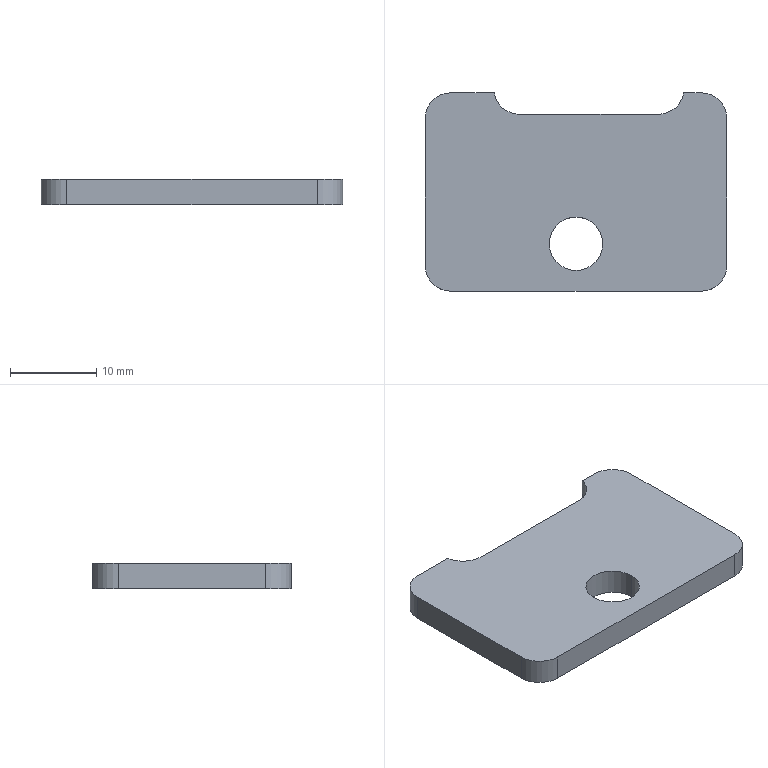Part | SolidWorks | features Fillet 2, MoveFace 2, Extrusion 1, ICE 1 | 1 solid | 16 faces | box 35 x 23 x 3 mm | volume 2147 mm3 | cylinder 8 | plane 8 | commonest cylinder face diameters 6 x6 6.2 x2
STEP:
#1=CARTESIAN_POINT('',(-3.1,-7.,3.));
#2=VERTEX_POINT('',#1);
#3=CARTESIAN_POINT('',(3.1,-7.,3.));
#4=VERTEX_POINT('',#3);
#5=CARTESIAN_POINT('',(0.,-7.,3.));
#6=DIRECTION('',(0.,0.,1.));
#7=DIRECTION('',(1.,0.,0.));
#8=AXIS2_PLACEMENT_3D('',#5,#6,#7);
#9=CIRCLE('',#8,3.1);
#10=EDGE_CURVE('',#2,#4,#9,.T.);
#11=ORIENTED_EDGE('',*,*,#10,.T.);
#12=CARTESIAN_POINT('',(3.1,-7.,0.));
#13=VERTEX_POINT('',#12);
#14=CARTESIAN_POINT('',(3.1,-7.,3.));
#15=DIRECTION('',(0.,0.,-1.));
#16=VECTOR('',#15,1000.);
#17=LINE('',#14,#16);
#18=EDGE_CURVE('',#4,#13,#17,.T.);
#19=ORIENTED_EDGE('',*,*,#18,.T.);
#20=CARTESIAN_POINT('',(-3.1,-7.,0.));
#21=VERTEX_POINT('',#20);
#22=CARTESIAN_POINT('',(0.,-7.,0.));
#23=DIRECTION('',(0.,0.,1.));
#24=DIRECTION('',(1.,0.,0.));
#25=AXIS2_PLACEMENT_3D('',#22,#23,#24);
#26=CIRCLE('',#25,3.1);
#27=EDGE_CURVE('',#21,#13,#26,.T.);
#28=ORIENTED_EDGE('',*,*,#27,.F.);
#29=CARTESIAN_POINT('',(-3.1,-7.,3.));
#30=DIRECTION('',(0.,0.,-1.));
#31=VECTOR('',#30,1000.);
#32=LINE('',#29,#31);
#33=EDGE_CURVE('',#2,#21,#32,.T.);
#34=ORIENTED_EDGE('',*,*,#33,.F.);
#35=EDGE_LOOP('',(#11,#19,#28,#34));
#36=FACE_OUTER_BOUND('',#35,.T.);
#37=CARTESIAN_POINT('',(0.,-7.,3.));
#38=DIRECTION('',(0.,0.,-1.));
#39=DIRECTION('',(-1.,0.,0.));
#40=AXIS2_PLACEMENT_3D('',#37,#38,#39);
#41=CYLINDRICAL_SURFACE('',#40,3.1);
#42=ADVANCED_FACE('',(#36),#41,.F.);
#43=CARTESIAN_POINT('',(-9.5,10.5,3.));
#44=VERTEX_POINT('',#43);
#45=CARTESIAN_POINT('',(-14.5,10.5,3.));
#46=VERTEX_POINT('',#45);
#47=CARTESIAN_POINT('',(-17.5,10.5,3.));
#48=DIRECTION('',(-1.,0.,0.));
#49=VECTOR('',#48,1000.);
#50=LINE('',#47,#49);
#51=EDGE_CURVE('',#44,#46,#50,.T.);
#52=ORIENTED_EDGE('',*,*,#51,.F.);
#53=CARTESIAN_POINT('',(-9.5,10.5,0.));
#54=VERTEX_POINT('',#53);
#55=CARTESIAN_POINT('',(-9.5,10.5,3.));
#56=DIRECTION('',(0.,0.,-1.));
#57=VECTOR('',#56,1000.);
#58=LINE('',#55,#57);
#59=EDGE_CURVE('',#44,#54,#58,.T.);
#60=ORIENTED_EDGE('',*,*,#59,.T.);
#61=CARTESIAN_POINT('',(-14.5,10.5,0.));
#62=VERTEX_POINT('',#61);
#63=CARTESIAN_POINT('',(-17.5,10.5,0.));
#64=DIRECTION('',(-1.,0.,0.));
#65=VECTOR('',#64,1000.);
#66=LINE('',#63,#65);
#67=EDGE_CURVE('',#54,#62,#66,.T.);
#68=ORIENTED_EDGE('',*,*,#67,.T.);
#69=CARTESIAN_POINT('',(-14.5,10.5,3.));
#70=DIRECTION('',(0.,0.,1.));
#71=VECTOR('',#70,1000.);
#72=LINE('',#69,#71);
#73=EDGE_CURVE('',#62,#46,#72,.T.);
#74=ORIENTED_EDGE('',*,*,#73,.T.);
#75=EDGE_LOOP('',(#52,#60,#68,#74));
#76=FACE_OUTER_BOUND('',#75,.T.);
#77=CARTESIAN_POINT('',(-17.5,10.5,3.));
#78=DIRECTION('',(0.,-1.,0.));
#79=DIRECTION('',(0.,0.,-1.));
#80=AXIS2_PLACEMENT_3D('',#77,#78,#79);
#81=PLANE('',#80);
#82=ADVANCED_FACE('',(#76),#81,.F.);
#83=CARTESIAN_POINT('',(9.542,8.,3.));
#84=VERTEX_POINT('',#83);
#85=CARTESIAN_POINT('',(-6.542,8.,3.));
#86=VERTEX_POINT('',#85);
#87=CARTESIAN_POINT('',(12.5,8.,3.));
#88=DIRECTION('',(-1.,0.,0.));
#89=VECTOR('',#88,1000.);
#90=LINE('',#87,#89);
#91=EDGE_CURVE('',#84,#86,#90,.T.);
#92=ORIENTED_EDGE('',*,*,#91,.T.);
#93=CARTESIAN_POINT('',(-6.542,11.,3.));
#94=DIRECTION('',(0.,0.,-1.));
#95=DIRECTION('',(1.,0.,0.));
#96=AXIS2_PLACEMENT_3D('',#93,#94,#95);
#97=CIRCLE('',#96,3.);
#98=EDGE_CURVE('',#86,#44,#97,.T.);
#99=ORIENTED_EDGE('',*,*,#98,.T.);
#100=ORIENTED_EDGE('',*,*,#51,.T.);
#101=CARTESIAN_POINT('',(-17.5,7.5,3.));
#102=VERTEX_POINT('',#101);
#103=CARTESIAN_POINT('',(-14.5,7.5,3.));
#104=DIRECTION('',(0.,0.,1.));
#105=DIRECTION('',(1.,0.,0.));
#106=AXIS2_PLACEMENT_3D('',#103,#104,#105);
#107=CIRCLE('',#106,3.);
#108=EDGE_CURVE('',#46,#102,#107,.T.);
#109=ORIENTED_EDGE('',*,*,#108,.T.);
#110=CARTESIAN_POINT('',(-17.5,-9.5,3.));
#111=VERTEX_POINT('',#110);
#112=CARTESIAN_POINT('',(-17.5,12.5,3.));
#113=DIRECTION('',(0.,-1.,0.));
#114=VECTOR('',#113,1000.);
#115=LINE('',#112,#114);
#116=EDGE_CURVE('',#102,#111,#115,.T.);
#117=ORIENTED_EDGE('',*,*,#116,.T.);
#118=CARTESIAN_POINT('',(-14.5,-12.5,3.));
#119=VERTEX_POINT('',#118);
#120=CARTESIAN_POINT('',(-14.5,-9.5,3.));
#121=DIRECTION('',(0.,0.,1.));
#122=DIRECTION('',(1.,0.,0.));
#123=AXIS2_PLACEMENT_3D('',#120,#121,#122);
#124=CIRCLE('',#123,3.);
#125=EDGE_CURVE('',#111,#119,#124,.T.);
#126=ORIENTED_EDGE('',*,*,#125,.T.);
#127=CARTESIAN_POINT('',(14.5,-12.5,3.));
#128=VERTEX_POINT('',#127);
#129=CARTESIAN_POINT('',(-17.5,-12.5,3.));
#130=DIRECTION('',(1.,0.,0.));
#131=VECTOR('',#130,1000.);
#132=LINE('',#129,#131);
#133=EDGE_CURVE('',#119,#128,#132,.T.);
#134=ORIENTED_EDGE('',*,*,#133,.T.);
#135=CARTESIAN_POINT('',(17.5,-9.5,3.));
#136=VERTEX_POINT('',#135);
#137=CARTESIAN_POINT('',(14.5,-9.5,3.));
#138=DIRECTION('',(0.,0.,1.));
#139=DIRECTION('',(1.,0.,0.));
#140=AXIS2_PLACEMENT_3D('',#137,#138,#139);
#141=CIRCLE('',#140,3.);
#142=EDGE_CURVE('',#128,#136,#141,.T.);
#143=ORIENTED_EDGE('',*,*,#142,.T.);
#144=CARTESIAN_POINT('',(17.5,7.5,3.));
#145=VERTEX_POINT('',#144);
#146=CARTESIAN_POINT('',(17.5,12.5,3.));
#147=DIRECTION('',(0.,1.,0.));
#148=VECTOR('',#147,1000.);
#149=LINE('',#146,#148);
#150=EDGE_CURVE('',#136,#145,#149,.T.);
#151=ORIENTED_EDGE('',*,*,#150,.T.);
#152=CARTESIAN_POINT('',(14.5,10.5,3.));
#153=VERTEX_POINT('',#152);
#154=CARTESIAN_POINT('',(14.5,7.5,3.));
#155=DIRECTION('',(0.,0.,1.));
#156=DIRECTION('',(1.,0.,0.));
#157=AXIS2_PLACEMENT_3D('',#154,#155,#156);
#158=CIRCLE('',#157,3.);
#159=EDGE_CURVE('',#145,#153,#158,.T.);
#160=ORIENTED_EDGE('',*,*,#159,.T.);
#161=CARTESIAN_POINT('',(12.5,10.5,3.));
#162=VERTEX_POINT('',#161);
#163=CARTESIAN_POINT('',(-17.5,10.5,3.));
#164=DIRECTION('',(-1.,0.,0.));
#165=VECTOR('',#164,1000.);
#166=LINE('',#163,#165);
#167=EDGE_CURVE('',#153,#162,#166,.T.);
#168=ORIENTED_EDGE('',*,*,#167,.T.);
#169=CARTESIAN_POINT('',(9.542,11.,3.));
#170=DIRECTION('',(0.,0.,-1.));
#171=DIRECTION('',(1.,0.,0.));
#172=AXIS2_PLACEMENT_3D('',#169,#170,#171);
#173=CIRCLE('',#172,3.);
#174=EDGE_CURVE('',#162,#84,#173,.T.);
#175=ORIENTED_EDGE('',*,*,#174,.T.);
#176=EDGE_LOOP('',(#92,#99,#100,#109,#117,#126,#134,#143,#151,#160,#168,#175));
#177=FACE_OUTER_BOUND('',#176,.T.);
#178=ORIENTED_EDGE('',*,*,#10,.F.);
#179=CARTESIAN_POINT('',(0.,-7.,3.));
#180=DIRECTION('',(0.,0.,1.));
#181=DIRECTION('',(1.,0.,0.));
#182=AXIS2_PLACEMENT_3D('',#179,#180,#181);
#183=CIRCLE('',#182,3.1);
#184=EDGE_CURVE('',#4,#2,#183,.T.);
#185=ORIENTED_EDGE('',*,*,#184,.F.);
#186=EDGE_LOOP('',(#178,#185));
#187=FACE_BOUND('',#186,.T.);
#188=CARTESIAN_POINT('',(0.,0.,3.));
#189=DIRECTION('',(0.,0.,1.));
#190=DIRECTION('',(1.,0.,0.));
#191=AXIS2_PLACEMENT_3D('',#188,#189,#190);
#192=PLANE('',#191);
#193=ADVANCED_FACE('',(#177,#187),#192,.T.);
#194=ORIENTED_EDGE('',*,*,#67,.F.);
#195=CARTESIAN_POINT('',(-6.542,8.,0.));
#196=VERTEX_POINT('',#195);
#197=CARTESIAN_POINT('',(-6.542,11.,0.));
#198=DIRECTION('',(0.,0.,1.));
#199=DIRECTION('',(1.,0.,0.));
#200=AXIS2_PLACEMENT_3D('',#197,#198,#199);
#201=CIRCLE('',#200,3.);
#202=EDGE_CURVE('',#54,#196,#201,.T.);
#203=ORIENTED_EDGE('',*,*,#202,.T.);
#204=CARTESIAN_POINT('',(9.542,8.,0.));
#205=VERTEX_POINT('',#204);
#206=CARTESIAN_POINT('',(12.5,8.,0.));
#207=DIRECTION('',(-1.,0.,0.));
#208=VECTOR('',#207,1000.);
#209=LINE('',#206,#208);
#210=EDGE_CURVE('',#205,#196,#209,.T.);
#211=ORIENTED_EDGE('',*,*,#210,.F.);
#212=CARTESIAN_POINT('',(12.5,10.5,0.));
#213=VERTEX_POINT('',#212);
#214=CARTESIAN_POINT('',(9.542,11.,0.));
#215=DIRECTION('',(0.,0.,1.));
#216=DIRECTION('',(1.,0.,0.));
#217=AXIS2_PLACEMENT_3D('',#214,#215,#216);
#218=CIRCLE('',#217,3.);
#219=EDGE_CURVE('',#205,#213,#218,.T.);
#220=ORIENTED_EDGE('',*,*,#219,.T.);
#221=CARTESIAN_POINT('',(14.5,10.5,0.));
#222=VERTEX_POINT('',#221);
#223=CARTESIAN_POINT('',(-17.5,10.5,0.));
#224=DIRECTION('',(-1.,0.,0.));
#225=VECTOR('',#224,1000.);
#226=LINE('',#223,#225);
#227=EDGE_CURVE('',#222,#213,#226,.T.);
#228=ORIENTED_EDGE('',*,*,#227,.F.);
#229=CARTESIAN_POINT('',(17.5,7.5,0.));
#230=VERTEX_POINT('',#229);
#231=CARTESIAN_POINT('',(14.5,7.5,0.));
#232=DIRECTION('',(0.,0.,-1.));
#233=DIRECTION('',(1.,0.,0.));
#234=AXIS2_PLACEMENT_3D('',#231,#232,#233);
#235=CIRCLE('',#234,3.);
#236=EDGE_CURVE('',#222,#230,#235,.T.);
#237=ORIENTED_EDGE('',*,*,#236,.T.);
#238=CARTESIAN_POINT('',(17.5,-9.5,0.));
#239=VERTEX_POINT('',#238);
#240=CARTESIAN_POINT('',(17.5,12.5,0.));
#241=DIRECTION('',(0.,1.,0.));
#242=VECTOR('',#241,1000.);
#243=LINE('',#240,#242);
#244=EDGE_CURVE('',#239,#230,#243,.T.);
#245=ORIENTED_EDGE('',*,*,#244,.F.);
#246=CARTESIAN_POINT('',(14.5,-12.5,0.));
#247=VERTEX_POINT('',#246);
#248=CARTESIAN_POINT('',(14.5,-9.5,0.));
#249=DIRECTION('',(0.,0.,-1.));
#250=DIRECTION('',(1.,0.,0.));
#251=AXIS2_PLACEMENT_3D('',#248,#249,#250);
#252=CIRCLE('',#251,3.);
#253=EDGE_CURVE('',#239,#247,#252,.T.);
#254=ORIENTED_EDGE('',*,*,#253,.T.);
#255=CARTESIAN_POINT('',(-14.5,-12.5,0.));
#256=VERTEX_POINT('',#255);
#257=CARTESIAN_POINT('',(-17.5,-12.5,0.));
#258=DIRECTION('',(1.,0.,0.));
#259=VECTOR('',#258,1000.);
#260=LINE('',#257,#259);
#261=EDGE_CURVE('',#256,#247,#260,.T.);
#262=ORIENTED_EDGE('',*,*,#261,.F.);
#263=CARTESIAN_POINT('',(-17.5,-9.5,0.));
#264=VERTEX_POINT('',#263);
#265=CARTESIAN_POINT('',(-14.5,-9.5,0.));
#266=DIRECTION('',(0.,0.,-1.));
#267=DIRECTION('',(1.,0.,0.));
#268=AXIS2_PLACEMENT_3D('',#265,#266,#267);
#269=CIRCLE('',#268,3.);
#270=EDGE_CURVE('',#256,#264,#269,.T.);
#271=ORIENTED_EDGE('',*,*,#270,.T.);
#272=CARTESIAN_POINT('',(-17.5,7.5,0.));
#273=VERTEX_POINT('',#272);
#274=CARTESIAN_POINT('',(-17.5,12.5,0.));
#275=DIRECTION('',(0.,-1.,0.));
#276=VECTOR('',#275,1000.);
#277=LINE('',#274,#276);
#278=EDGE_CURVE('',#273,#264,#277,.T.);
#279=ORIENTED_EDGE('',*,*,#278,.F.);
#280=CARTESIAN_POINT('',(-14.5,7.5,0.));
#281=DIRECTION('',(0.,0.,-1.));
#282=DIRECTION('',(1.,0.,0.));
#283=AXIS2_PLACEMENT_3D('',#280,#281,#282);
#284=CIRCLE('',#283,3.);
#285=EDGE_CURVE('',#273,#62,#284,.T.);
#286=ORIENTED_EDGE('',*,*,#285,.T.);
#287=EDGE_LOOP('',(#194,#203,#211,#220,#228,#237,#245,#254,#262,#271,#279,#286));
#288=FACE_OUTER_BOUND('',#287,.T.);
#289=ORIENTED_EDGE('',*,*,#27,.T.);
#290=CARTESIAN_POINT('',(0.,-7.,0.));
#291=DIRECTION('',(0.,0.,1.));
#292=DIRECTION('',(1.,0.,0.));
#293=AXIS2_PLACEMENT_3D('',#290,#291,#292);
#294=CIRCLE('',#293,3.1);
#295=EDGE_CURVE('',#13,#21,#294,.T.);
#296=ORIENTED_EDGE('',*,*,#295,.T.);
#297=EDGE_LOOP('',(#289,#296));
#298=FACE_BOUND('',#297,.T.);
#299=CARTESIAN_POINT('',(0.,0.,0.));
#300=DIRECTION('',(0.,0.,1.));
#301=DIRECTION('',(1.,0.,0.));
#302=AXIS2_PLACEMENT_3D('',#299,#300,#301);
#303=PLANE('',#302);
#304=ADVANCED_FACE('',(#288,#298),#303,.F.);
#305=ORIENTED_EDGE('',*,*,#244,.T.);
#306=CARTESIAN_POINT('',(17.5,7.5,3.));
#307=DIRECTION('',(0.,0.,1.));
#308=VECTOR('',#307,1000.);
#309=LINE('',#306,#308);
#310=EDGE_CURVE('',#230,#145,#309,.T.);
#311=ORIENTED_EDGE('',*,*,#310,.T.);
#312=ORIENTED_EDGE('',*,*,#150,.F.);
#313=CARTESIAN_POINT('',(17.5,-9.5,3.));
#314=DIRECTION('',(0.,0.,-1.));
#315=VECTOR('',#314,1000.);
#316=LINE('',#313,#315);
#317=EDGE_CURVE('',#136,#239,#316,.T.);
#318=ORIENTED_EDGE('',*,*,#317,.T.);
#319=EDGE_LOOP('',(#305,#311,#312,#318));
#320=FACE_OUTER_BOUND('',#319,.T.);
#321=CARTESIAN_POINT('',(17.5,12.5,3.));
#322=DIRECTION('',(-1.,0.,0.));
#323=DIRECTION('',(0.,-1.,0.));
#324=AXIS2_PLACEMENT_3D('',#321,#322,#323);
#325=PLANE('',#324);
#326=ADVANCED_FACE('',(#320),#325,.F.);
#327=ORIENTED_EDGE('',*,*,#227,.T.);
#328=CARTESIAN_POINT('',(12.5,10.5,3.));
#329=DIRECTION('',(0.,0.,1.));
#330=VECTOR('',#329,1000.);
#331=LINE('',#328,#330);
#332=EDGE_CURVE('',#213,#162,#331,.T.);
#333=ORIENTED_EDGE('',*,*,#332,.T.);
#334=ORIENTED_EDGE('',*,*,#167,.F.);
#335=CARTESIAN_POINT('',(14.5,10.5,3.));
#336=DIRECTION('',(0.,0.,-1.));
#337=VECTOR('',#336,1000.);
#338=LINE('',#335,#337);
#339=EDGE_CURVE('',#153,#222,#338,.T.);
#340=ORIENTED_EDGE('',*,*,#339,.T.);
#341=EDGE_LOOP('',(#327,#333,#334,#340));
#342=FACE_OUTER_BOUND('',#341,.T.);
#343=CARTESIAN_POINT('',(-17.5,10.5,3.));
#344=DIRECTION('',(0.,-1.,0.));
#345=DIRECTION('',(0.,0.,-1.));
#346=AXIS2_PLACEMENT_3D('',#343,#344,#345);
#347=PLANE('',#346);
#348=ADVANCED_FACE('',(#342),#347,.F.);
#349=ORIENTED_EDGE('',*,*,#278,.T.);
#350=CARTESIAN_POINT('',(-17.5,-9.5,3.));
#351=DIRECTION('',(0.,0.,1.));
#352=VECTOR('',#351,1000.);
#353=LINE('',#350,#352);
#354=EDGE_CURVE('',#264,#111,#353,.T.);
#355=ORIENTED_EDGE('',*,*,#354,.T.);
#356=ORIENTED_EDGE('',*,*,#116,.F.);
#357=CARTESIAN_POINT('',(-17.5,7.5,3.));
#358=DIRECTION('',(0.,0.,-1.));
#359=VECTOR('',#358,1000.);
#360=LINE('',#357,#359);
#361=EDGE_CURVE('',#102,#273,#360,.T.);
#362=ORIENTED_EDGE('',*,*,#361,.T.);
#363=EDGE_LOOP('',(#349,#355,#356,#362));
#364=FACE_OUTER_BOUND('',#363,.T.);
#365=CARTESIAN_POINT('',(-17.5,12.5,3.));
#366=DIRECTION('',(1.,0.,0.));
#367=DIRECTION('',(0.,1.,0.));
#368=AXIS2_PLACEMENT_3D('',#365,#366,#367);
#369=PLANE('',#368);
#370=ADVANCED_FACE('',(#364),#369,.F.);
#371=ORIENTED_EDGE('',*,*,#261,.T.);
#372=CARTESIAN_POINT('',(14.5,-12.5,3.));
#373=DIRECTION('',(0.,0.,1.));
#374=VECTOR('',#373,1000.);
#375=LINE('',#372,#374);
#376=EDGE_CURVE('',#247,#128,#375,.T.);
#377=ORIENTED_EDGE('',*,*,#376,.T.);
#378=ORIENTED_EDGE('',*,*,#133,.F.);
#379=CARTESIAN_POINT('',(-14.5,-12.5,3.));
#380=DIRECTION('',(0.,0.,-1.));
#381=VECTOR('',#380,1000.);
#382=LINE('',#379,#381);
#383=EDGE_CURVE('',#119,#256,#382,.T.);
#384=ORIENTED_EDGE('',*,*,#383,.T.);
#385=EDGE_LOOP('',(#371,#377,#378,#384));
#386=FACE_OUTER_BOUND('',#385,.T.);
#387=CARTESIAN_POINT('',(-17.5,-12.5,3.));
#388=DIRECTION('',(0.,1.,0.));
#389=DIRECTION('',(0.,0.,1.));
#390=AXIS2_PLACEMENT_3D('',#387,#388,#389);
#391=PLANE('',#390);
#392=ADVANCED_FACE('',(#386),#391,.F.);
#393=ORIENTED_EDGE('',*,*,#18,.F.);
#394=ORIENTED_EDGE('',*,*,#184,.T.);
#395=ORIENTED_EDGE('',*,*,#33,.T.);
#396=ORIENTED_EDGE('',*,*,#295,.F.);
#397=EDGE_LOOP('',(#393,#394,#395,#396));
#398=FACE_OUTER_BOUND('',#397,.T.);
#399=CARTESIAN_POINT('',(0.,-7.,3.));
#400=DIRECTION('',(0.,0.,-1.));
#401=DIRECTION('',(-1.,0.,0.));
#402=AXIS2_PLACEMENT_3D('',#399,#400,#401);
#403=CYLINDRICAL_SURFACE('',#402,3.1);
#404=ADVANCED_FACE('',(#398),#403,.F.);
#405=ORIENTED_EDGE('',*,*,#159,.F.);
#406=ORIENTED_EDGE('',*,*,#310,.F.);
#407=ORIENTED_EDGE('',*,*,#236,.F.);
#408=ORIENTED_EDGE('',*,*,#339,.F.);
#409=EDGE_LOOP('',(#405,#406,#407,#408));
#410=FACE_OUTER_BOUND('',#409,.T.);
#411=CARTESIAN_POINT('',(14.5,7.5,3.));
#412=DIRECTION('',(0.,0.,-1.));
#413=DIRECTION('',(-1.,0.,0.));
#414=AXIS2_PLACEMENT_3D('',#411,#412,#413);
#415=CYLINDRICAL_SURFACE('',#414,3.);
#416=ADVANCED_FACE('',(#410),#415,.T.);
#417=ORIENTED_EDGE('',*,*,#142,.F.);
#418=ORIENTED_EDGE('',*,*,#376,.F.);
#419=ORIENTED_EDGE('',*,*,#253,.F.);
#420=ORIENTED_EDGE('',*,*,#317,.F.);
#421=EDGE_LOOP('',(#417,#418,#419,#420));
#422=FACE_OUTER_BOUND('',#421,.T.);
#423=CARTESIAN_POINT('',(14.5,-9.5,3.));
#424=DIRECTION('',(0.,0.,-1.));
#425=DIRECTION('',(-1.,0.,0.));
#426=AXIS2_PLACEMENT_3D('',#423,#424,#425);
#427=CYLINDRICAL_SURFACE('',#426,3.);
#428=ADVANCED_FACE('',(#422),#427,.T.);
#429=ORIENTED_EDGE('',*,*,#125,.F.);
#430=ORIENTED_EDGE('',*,*,#354,.F.);
#431=ORIENTED_EDGE('',*,*,#270,.F.);
#432=ORIENTED_EDGE('',*,*,#383,.F.);
#433=EDGE_LOOP('',(#429,#430,#431,#432));
#434=FACE_OUTER_BOUND('',#433,.T.);
#435=CARTESIAN_POINT('',(-14.5,-9.5,3.));
#436=DIRECTION('',(0.,0.,-1.));
#437=DIRECTION('',(-1.,0.,0.));
#438=AXIS2_PLACEMENT_3D('',#435,#436,#437);
#439=CYLINDRICAL_SURFACE('',#438,3.);
#440=ADVANCED_FACE('',(#434),#439,.T.);
#441=ORIENTED_EDGE('',*,*,#108,.F.);
#442=ORIENTED_EDGE('',*,*,#73,.F.);
#443=ORIENTED_EDGE('',*,*,#285,.F.);
#444=ORIENTED_EDGE('',*,*,#361,.F.);
#445=EDGE_LOOP('',(#441,#442,#443,#444));
#446=FACE_OUTER_BOUND('',#445,.T.);
#447=CARTESIAN_POINT('',(-14.5,7.5,3.));
#448=DIRECTION('',(0.,0.,-1.));
#449=DIRECTION('',(-1.,0.,0.));
#450=AXIS2_PLACEMENT_3D('',#447,#448,#449);
#451=CYLINDRICAL_SURFACE('',#450,3.);
#452=ADVANCED_FACE('',(#446),#451,.T.);
#453=ORIENTED_EDGE('',*,*,#210,.T.);
#454=CARTESIAN_POINT('',(-6.542,8.,3.));
#455=DIRECTION('',(0.,0.,1.));
#456=VECTOR('',#455,1000.);
#457=LINE('',#454,#456);
#458=EDGE_CURVE('',#196,#86,#457,.T.);
#459=ORIENTED_EDGE('',*,*,#458,.T.);
#460=ORIENTED_EDGE('',*,*,#91,.F.);
#461=CARTESIAN_POINT('',(9.542,8.,3.));
#462=DIRECTION('',(0.,0.,-1.));
#463=VECTOR('',#462,1000.);
#464=LINE('',#461,#463);
#465=EDGE_CURVE('',#84,#205,#464,.T.);
#466=ORIENTED_EDGE('',*,*,#465,.T.);
#467=EDGE_LOOP('',(#453,#459,#460,#466));
#468=FACE_OUTER_BOUND('',#467,.T.);
#469=CARTESIAN_POINT('',(12.5,8.,3.));
#470=DIRECTION('',(0.,-1.,0.));
#471=DIRECTION('',(0.,0.,-1.));
#472=AXIS2_PLACEMENT_3D('',#469,#470,#471);
#473=PLANE('',#472);
#474=ADVANCED_FACE('',(#468),#473,.F.);
#475=ORIENTED_EDGE('',*,*,#98,.F.);
#476=ORIENTED_EDGE('',*,*,#458,.F.);
#477=ORIENTED_EDGE('',*,*,#202,.F.);
#478=ORIENTED_EDGE('',*,*,#59,.F.);
#479=EDGE_LOOP('',(#475,#476,#477,#478));
#480=FACE_OUTER_BOUND('',#479,.T.);
#481=CARTESIAN_POINT('',(-6.542,11.,3.));
#482=DIRECTION('',(0.,0.,1.));
#483=DIRECTION('',(1.,0.,0.));
#484=AXIS2_PLACEMENT_3D('',#481,#482,#483);
#485=CYLINDRICAL_SURFACE('',#484,3.);
#486=ADVANCED_FACE('',(#480),#485,.F.);
#487=ORIENTED_EDGE('',*,*,#174,.F.);
#488=ORIENTED_EDGE('',*,*,#332,.F.);
#489=ORIENTED_EDGE('',*,*,#219,.F.);
#490=ORIENTED_EDGE('',*,*,#465,.F.);
#491=EDGE_LOOP('',(#487,#488,#489,#490));
#492=FACE_OUTER_BOUND('',#491,.T.);
#493=CARTESIAN_POINT('',(9.542,11.,3.));
#494=DIRECTION('',(0.,0.,-1.));
#495=DIRECTION('',(-1.,0.,0.));
#496=AXIS2_PLACEMENT_3D('',#493,#494,#495);
#497=CYLINDRICAL_SURFACE('',#496,3.);
#498=ADVANCED_FACE('',(#492),#497,.F.);
#499=CLOSED_SHELL('',(#42,#82,#193,#304,#326,#348,#370,#392,#404,#416,#428,#440,#452,#474,#486,#498));
#500=MANIFOLD_SOLID_BREP('',#499);
#501=CARTESIAN_POINT('',(0.,0.,0.));
#502=DIRECTION('',(0.,0.,1.));
#503=DIRECTION('',(1.,0.,0.));
#504=AXIS2_PLACEMENT_3D('',#501,#502,#503);
#505=(LENGTH_UNIT()NAMED_UNIT(*)SI_UNIT(.MILLI.,.METRE.));
#506=UNCERTAINTY_MEASURE_WITH_UNIT(LENGTH_MEASURE(0.00001),#505,'','');
#507=(NAMED_UNIT(*)PLANE_ANGLE_UNIT()SI_UNIT($,.RADIAN.));
#508=(NAMED_UNIT(*)SI_UNIT($,.STERADIAN.)SOLID_ANGLE_UNIT());
#509=(GEOMETRIC_REPRESENTATION_CONTEXT(3)GLOBAL_UNCERTAINTY_ASSIGNED_CONTEXT((#506))GLOBAL_UNIT_ASSIGNED_CONTEXT((#505,#507,#508))REPRESENTATION_CONTEXT('',''));
#510=ADVANCED_BREP_SHAPE_REPRESENTATION('',(#500,#504),#509);